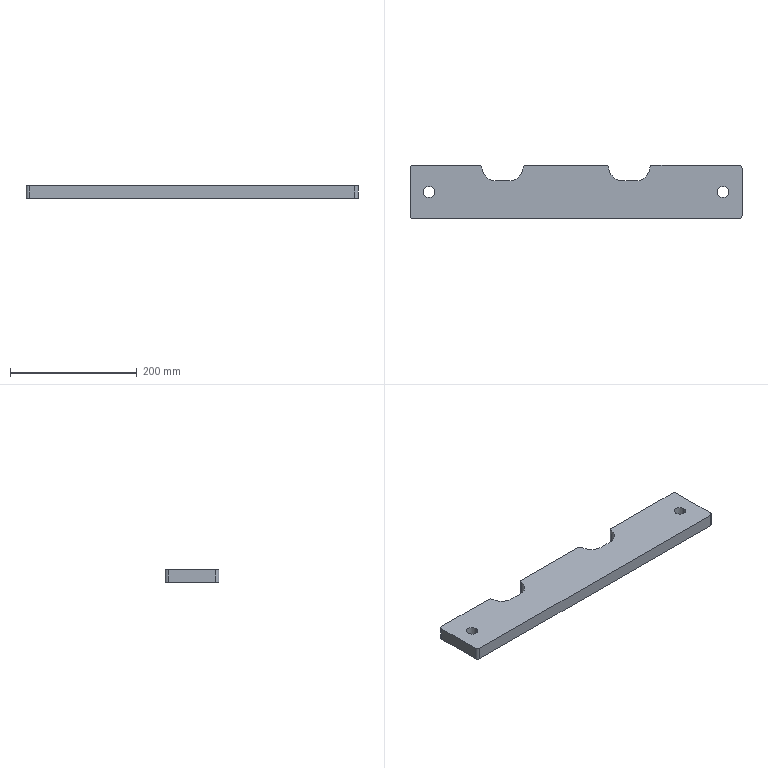Part | SolidWorks | features Extrusion 1 | 1 solid | 26 faces | box 524 x 85 x 20 mm | volume 823491 mm3 | cylinder 16 | plane 10 | commonest cylinder face diameters 10 x8 18 x4 45 x4
STEP:
#1=CARTESIAN_POINT('',(-26200.045,9505.463,20.));
#2=VERTEX_POINT('',#1);
#3=CARTESIAN_POINT('',(-26182.045,9505.463,20.));
#4=VERTEX_POINT('',#3);
#5=CARTESIAN_POINT('',(-26191.045,9505.463,20.));
#6=DIRECTION('',(0.,0.,1.));
#7=DIRECTION('',(1.,0.,0.));
#8=AXIS2_PLACEMENT_3D('',#5,#6,#7);
#9=CIRCLE('',#8,9.);
#10=EDGE_CURVE('',#2,#4,#9,.T.);
#11=ORIENTED_EDGE('',*,*,#10,.T.);
#12=CARTESIAN_POINT('',(-26182.045,9505.463,0.));
#13=VERTEX_POINT('',#12);
#14=CARTESIAN_POINT('',(-26182.045,9505.463,20.));
#15=DIRECTION('',(0.,0.,-1.));
#16=VECTOR('',#15,1000.);
#17=LINE('',#14,#16);
#18=EDGE_CURVE('',#4,#13,#17,.T.);
#19=ORIENTED_EDGE('',*,*,#18,.T.);
#20=CARTESIAN_POINT('',(-26200.045,9505.463,0.));
#21=VERTEX_POINT('',#20);
#22=CARTESIAN_POINT('',(-26191.045,9505.463,0.));
#23=DIRECTION('',(0.,0.,1.));
#24=DIRECTION('',(1.,0.,0.));
#25=AXIS2_PLACEMENT_3D('',#22,#23,#24);
#26=CIRCLE('',#25,9.);
#27=EDGE_CURVE('',#21,#13,#26,.T.);
#28=ORIENTED_EDGE('',*,*,#27,.F.);
#29=CARTESIAN_POINT('',(-26200.045,9505.463,20.));
#30=DIRECTION('',(0.,0.,-1.));
#31=VECTOR('',#30,1000.);
#32=LINE('',#29,#31);
#33=EDGE_CURVE('',#2,#21,#32,.T.);
#34=ORIENTED_EDGE('',*,*,#33,.F.);
#35=EDGE_LOOP('',(#11,#19,#28,#34));
#36=FACE_OUTER_BOUND('',#35,.T.);
#37=CARTESIAN_POINT('',(-26191.045,9505.463,20.));
#38=DIRECTION('',(0.,0.,-1.));
#39=DIRECTION('',(-1.,0.,0.));
#40=AXIS2_PLACEMENT_3D('',#37,#38,#39);
#41=CYLINDRICAL_SURFACE('',#40,9.);
#42=ADVANCED_FACE('',(#36),#41,.F.);
#43=CARTESIAN_POINT('',(-26664.045,9505.463,20.));
#44=VERTEX_POINT('',#43);
#45=CARTESIAN_POINT('',(-26646.045,9505.463,20.));
#46=VERTEX_POINT('',#45);
#47=CARTESIAN_POINT('',(-26655.045,9505.463,20.));
#48=DIRECTION('',(0.,0.,1.));
#49=DIRECTION('',(1.,0.,0.));
#50=AXIS2_PLACEMENT_3D('',#47,#48,#49);
#51=CIRCLE('',#50,9.);
#52=EDGE_CURVE('',#44,#46,#51,.T.);
#53=ORIENTED_EDGE('',*,*,#52,.T.);
#54=CARTESIAN_POINT('',(-26646.045,9505.463,0.));
#55=VERTEX_POINT('',#54);
#56=CARTESIAN_POINT('',(-26646.045,9505.463,20.));
#57=DIRECTION('',(0.,0.,-1.));
#58=VECTOR('',#57,1000.);
#59=LINE('',#56,#58);
#60=EDGE_CURVE('',#46,#55,#59,.T.);
#61=ORIENTED_EDGE('',*,*,#60,.T.);
#62=CARTESIAN_POINT('',(-26664.045,9505.463,0.));
#63=VERTEX_POINT('',#62);
#64=CARTESIAN_POINT('',(-26655.045,9505.463,0.));
#65=DIRECTION('',(0.,0.,1.));
#66=DIRECTION('',(1.,0.,0.));
#67=AXIS2_PLACEMENT_3D('',#64,#65,#66);
#68=CIRCLE('',#67,9.);
#69=EDGE_CURVE('',#63,#55,#68,.T.);
#70=ORIENTED_EDGE('',*,*,#69,.F.);
#71=CARTESIAN_POINT('',(-26664.045,9505.463,20.));
#72=DIRECTION('',(0.,0.,-1.));
#73=VECTOR('',#72,1000.);
#74=LINE('',#71,#73);
#75=EDGE_CURVE('',#44,#63,#74,.T.);
#76=ORIENTED_EDGE('',*,*,#75,.F.);
#77=EDGE_LOOP('',(#53,#61,#70,#76));
#78=FACE_OUTER_BOUND('',#77,.T.);
#79=CARTESIAN_POINT('',(-26655.045,9505.463,20.));
#80=DIRECTION('',(0.,0.,-1.));
#81=DIRECTION('',(-1.,0.,0.));
#82=AXIS2_PLACEMENT_3D('',#79,#80,#81);
#83=CYLINDRICAL_SURFACE('',#82,9.);
#84=ADVANCED_FACE('',(#78),#83,.F.);
#85=ORIENTED_EDGE('',*,*,#52,.F.);
#86=CARTESIAN_POINT('',(-26655.045,9505.463,20.));
#87=DIRECTION('',(0.,0.,1.));
#88=DIRECTION('',(1.,0.,0.));
#89=AXIS2_PLACEMENT_3D('',#86,#87,#88);
#90=CIRCLE('',#89,9.);
#91=EDGE_CURVE('',#46,#44,#90,.T.);
#92=ORIENTED_EDGE('',*,*,#91,.F.);
#93=EDGE_LOOP('',(#85,#92));
#94=FACE_BOUND('',#93,.T.);
#95=CARTESIAN_POINT('',(-26501.659,9547.963,20.));
#96=VERTEX_POINT('',#95);
#97=CARTESIAN_POINT('',(-26506.639,9543.418,20.));
#98=VERTEX_POINT('',#97);
#99=CARTESIAN_POINT('',(-26501.659,9542.963,20.));
#100=DIRECTION('',(0.,0.,1.));
#101=DIRECTION('',(1.,0.,0.));
#102=AXIS2_PLACEMENT_3D('',#99,#100,#101);
#103=CIRCLE('',#102,5.);
#104=EDGE_CURVE('',#96,#98,#103,.T.);
#105=ORIENTED_EDGE('',*,*,#104,.T.);
#106=CARTESIAN_POINT('',(-26529.045,9522.963,20.));
#107=VERTEX_POINT('',#106);
#108=CARTESIAN_POINT('',(-26529.045,9545.463,20.));
#109=DIRECTION('',(0.,0.,-1.));
#110=DIRECTION('',(1.,0.,0.));
#111=AXIS2_PLACEMENT_3D('',#108,#109,#110);
#112=CIRCLE('',#111,22.5);
#113=EDGE_CURVE('',#98,#107,#112,.T.);
#114=ORIENTED_EDGE('',*,*,#113,.T.);
#115=CARTESIAN_POINT('',(-26549.045,9522.963,20.));
#116=VERTEX_POINT('',#115);
#117=CARTESIAN_POINT('',(-26549.045,9522.963,20.));
#118=DIRECTION('',(-1.,0.,0.));
#119=VECTOR('',#118,1000.);
#120=LINE('',#117,#119);
#121=EDGE_CURVE('',#107,#116,#120,.T.);
#122=ORIENTED_EDGE('',*,*,#121,.T.);
#123=CARTESIAN_POINT('',(-26571.452,9543.418,20.));
#124=VERTEX_POINT('',#123);
#125=CARTESIAN_POINT('',(-26549.045,9545.463,20.));
#126=DIRECTION('',(0.,0.,-1.));
#127=DIRECTION('',(1.,0.,0.));
#128=AXIS2_PLACEMENT_3D('',#125,#126,#127);
#129=CIRCLE('',#128,22.5);
#130=EDGE_CURVE('',#116,#124,#129,.T.);
#131=ORIENTED_EDGE('',*,*,#130,.T.);
#132=CARTESIAN_POINT('',(-26576.432,9547.963,20.));
#133=VERTEX_POINT('',#132);
#134=CARTESIAN_POINT('',(-26576.432,9542.963,20.));
#135=DIRECTION('',(0.,0.,1.));
#136=DIRECTION('',(1.,0.,0.));
#137=AXIS2_PLACEMENT_3D('',#134,#135,#136);
#138=CIRCLE('',#137,5.);
#139=EDGE_CURVE('',#124,#133,#138,.T.);
#140=ORIENTED_EDGE('',*,*,#139,.T.);
#141=CARTESIAN_POINT('',(-26680.045,9547.963,20.));
#142=VERTEX_POINT('',#141);
#143=CARTESIAN_POINT('',(-26680.045,9547.963,20.));
#144=DIRECTION('',(-1.,0.,0.));
#145=VECTOR('',#144,1000.);
#146=LINE('',#143,#145);
#147=EDGE_CURVE('',#133,#142,#146,.T.);
#148=ORIENTED_EDGE('',*,*,#147,.T.);
#149=CARTESIAN_POINT('',(-26685.045,9542.963,20.));
#150=VERTEX_POINT('',#149);
#151=CARTESIAN_POINT('',(-26680.045,9542.963,20.));
#152=DIRECTION('',(0.,0.,1.));
#153=DIRECTION('',(1.,0.,0.));
#154=AXIS2_PLACEMENT_3D('',#151,#152,#153);
#155=CIRCLE('',#154,5.);
#156=EDGE_CURVE('',#142,#150,#155,.T.);
#157=ORIENTED_EDGE('',*,*,#156,.T.);
#158=CARTESIAN_POINT('',(-26685.045,9467.963,20.));
#159=VERTEX_POINT('',#158);
#160=CARTESIAN_POINT('',(-26685.045,9467.963,20.));
#161=DIRECTION('',(0.,-1.,0.));
#162=VECTOR('',#161,1000.);
#163=LINE('',#160,#162);
#164=EDGE_CURVE('',#150,#159,#163,.T.);
#165=ORIENTED_EDGE('',*,*,#164,.T.);
#166=CARTESIAN_POINT('',(-26680.045,9462.963,20.));
#167=VERTEX_POINT('',#166);
#168=CARTESIAN_POINT('',(-26680.045,9467.963,20.));
#169=DIRECTION('',(0.,0.,1.));
#170=DIRECTION('',(1.,0.,0.));
#171=AXIS2_PLACEMENT_3D('',#168,#169,#170);
#172=CIRCLE('',#171,5.);
#173=EDGE_CURVE('',#159,#167,#172,.T.);
#174=ORIENTED_EDGE('',*,*,#173,.T.);
#175=CARTESIAN_POINT('',(-26166.045,9462.963,20.));
#176=VERTEX_POINT('',#175);
#177=CARTESIAN_POINT('',(-26166.045,9462.963,20.));
#178=DIRECTION('',(1.,0.,0.));
#179=VECTOR('',#178,1000.);
#180=LINE('',#177,#179);
#181=EDGE_CURVE('',#167,#176,#180,.T.);
#182=ORIENTED_EDGE('',*,*,#181,.T.);
#183=CARTESIAN_POINT('',(-26161.045,9467.963,20.));
#184=VERTEX_POINT('',#183);
#185=CARTESIAN_POINT('',(-26166.045,9467.963,20.));
#186=DIRECTION('',(0.,0.,1.));
#187=DIRECTION('',(1.,0.,0.));
#188=AXIS2_PLACEMENT_3D('',#185,#186,#187);
#189=CIRCLE('',#188,5.);
#190=EDGE_CURVE('',#176,#184,#189,.T.);
#191=ORIENTED_EDGE('',*,*,#190,.T.);
#192=CARTESIAN_POINT('',(-26161.045,9542.963,20.));
#193=VERTEX_POINT('',#192);
#194=CARTESIAN_POINT('',(-26161.045,9467.963,20.));
#195=DIRECTION('',(0.,1.,0.));
#196=VECTOR('',#195,1000.);
#197=LINE('',#194,#196);
#198=EDGE_CURVE('',#184,#193,#197,.T.);
#199=ORIENTED_EDGE('',*,*,#198,.T.);
#200=CARTESIAN_POINT('',(-26166.045,9547.963,20.));
#201=VERTEX_POINT('',#200);
#202=CARTESIAN_POINT('',(-26166.045,9542.963,20.));
#203=DIRECTION('',(0.,0.,1.));
#204=DIRECTION('',(1.,0.,0.));
#205=AXIS2_PLACEMENT_3D('',#202,#203,#204);
#206=CIRCLE('',#205,5.);
#207=EDGE_CURVE('',#193,#201,#206,.T.);
#208=ORIENTED_EDGE('',*,*,#207,.T.);
#209=CARTESIAN_POINT('',(-26301.659,9547.963,20.));
#210=VERTEX_POINT('',#209);
#211=CARTESIAN_POINT('',(-26289.045,9547.963,20.));
#212=DIRECTION('',(-1.,0.,0.));
#213=VECTOR('',#212,1000.);
#214=LINE('',#211,#213);
#215=EDGE_CURVE('',#201,#210,#214,.T.);
#216=ORIENTED_EDGE('',*,*,#215,.T.);
#217=CARTESIAN_POINT('',(-26306.639,9543.418,20.));
#218=VERTEX_POINT('',#217);
#219=CARTESIAN_POINT('',(-26301.659,9542.963,20.));
#220=DIRECTION('',(0.,0.,1.));
#221=DIRECTION('',(1.,0.,0.));
#222=AXIS2_PLACEMENT_3D('',#219,#220,#221);
#223=CIRCLE('',#222,5.);
#224=EDGE_CURVE('',#210,#218,#223,.T.);
#225=ORIENTED_EDGE('',*,*,#224,.T.);
#226=CARTESIAN_POINT('',(-26329.045,9522.963,20.));
#227=VERTEX_POINT('',#226);
#228=CARTESIAN_POINT('',(-26329.045,9545.463,20.));
#229=DIRECTION('',(0.,0.,-1.));
#230=DIRECTION('',(1.,0.,0.));
#231=AXIS2_PLACEMENT_3D('',#228,#229,#230);
#232=CIRCLE('',#231,22.5);
#233=EDGE_CURVE('',#218,#227,#232,.T.);
#234=ORIENTED_EDGE('',*,*,#233,.T.);
#235=CARTESIAN_POINT('',(-26349.045,9522.963,20.));
#236=VERTEX_POINT('',#235);
#237=CARTESIAN_POINT('',(-26349.045,9522.963,20.));
#238=DIRECTION('',(-1.,0.,0.));
#239=VECTOR('',#238,1000.);
#240=LINE('',#237,#239);
#241=EDGE_CURVE('',#227,#236,#240,.T.);
#242=ORIENTED_EDGE('',*,*,#241,.T.);
#243=CARTESIAN_POINT('',(-26371.452,9543.418,20.));
#244=VERTEX_POINT('',#243);
#245=CARTESIAN_POINT('',(-26349.045,9545.463,20.));
#246=DIRECTION('',(0.,0.,-1.));
#247=DIRECTION('',(1.,0.,0.));
#248=AXIS2_PLACEMENT_3D('',#245,#246,#247);
#249=CIRCLE('',#248,22.5);
#250=EDGE_CURVE('',#236,#244,#249,.T.);
#251=ORIENTED_EDGE('',*,*,#250,.T.);
#252=CARTESIAN_POINT('',(-26376.432,9547.963,20.));
#253=VERTEX_POINT('',#252);
#254=CARTESIAN_POINT('',(-26376.432,9542.963,20.));
#255=DIRECTION('',(0.,0.,1.));
#256=DIRECTION('',(1.,0.,0.));
#257=AXIS2_PLACEMENT_3D('',#254,#255,#256);
#258=CIRCLE('',#257,5.);
#259=EDGE_CURVE('',#244,#253,#258,.T.);
#260=ORIENTED_EDGE('',*,*,#259,.T.);
#261=CARTESIAN_POINT('',(-26501.659,9547.963,20.));
#262=DIRECTION('',(-1.,0.,0.));
#263=VECTOR('',#262,1000.);
#264=LINE('',#261,#263);
#265=EDGE_CURVE('',#253,#96,#264,.T.);
#266=ORIENTED_EDGE('',*,*,#265,.T.);
#267=EDGE_LOOP('',(#105,#114,#122,#131,#140,#148,#157,#165,#174,#182,#191,#199,#208,#216,#225,#234,#242,#251,#260,#266));
#268=FACE_OUTER_BOUND('',#267,.T.);
#269=ORIENTED_EDGE('',*,*,#10,.F.);
#270=CARTESIAN_POINT('',(-26191.045,9505.463,20.));
#271=DIRECTION('',(0.,0.,1.));
#272=DIRECTION('',(1.,0.,0.));
#273=AXIS2_PLACEMENT_3D('',#270,#271,#272);
#274=CIRCLE('',#273,9.);
#275=EDGE_CURVE('',#4,#2,#274,.T.);
#276=ORIENTED_EDGE('',*,*,#275,.F.);
#277=EDGE_LOOP('',(#269,#276));
#278=FACE_BOUND('',#277,.T.);
#279=CARTESIAN_POINT('',(-26501.659,9542.963,20.));
#280=DIRECTION('',(0.,0.,1.));
#281=DIRECTION('',(1.,0.,0.));
#282=AXIS2_PLACEMENT_3D('',#279,#280,#281);
#283=PLANE('',#282);
#284=ADVANCED_FACE('',(#94,#268,#278),#283,.T.);
#285=CARTESIAN_POINT('',(-26501.659,9547.963,0.));
#286=VERTEX_POINT('',#285);
#287=CARTESIAN_POINT('',(-26506.639,9543.418,0.));
#288=VERTEX_POINT('',#287);
#289=CARTESIAN_POINT('',(-26501.659,9542.963,0.));
#290=DIRECTION('',(0.,0.,1.));
#291=DIRECTION('',(1.,0.,0.));
#292=AXIS2_PLACEMENT_3D('',#289,#290,#291);
#293=CIRCLE('',#292,5.);
#294=EDGE_CURVE('',#286,#288,#293,.T.);
#295=ORIENTED_EDGE('',*,*,#294,.F.);
#296=CARTESIAN_POINT('',(-26376.432,9547.963,0.));
#297=VERTEX_POINT('',#296);
#298=CARTESIAN_POINT('',(-26501.659,9547.963,0.));
#299=DIRECTION('',(-1.,0.,0.));
#300=VECTOR('',#299,1000.);
#301=LINE('',#298,#300);
#302=EDGE_CURVE('',#297,#286,#301,.T.);
#303=ORIENTED_EDGE('',*,*,#302,.F.);
#304=CARTESIAN_POINT('',(-26371.452,9543.418,0.));
#305=VERTEX_POINT('',#304);
#306=CARTESIAN_POINT('',(-26376.432,9542.963,0.));
#307=DIRECTION('',(0.,0.,1.));
#308=DIRECTION('',(1.,0.,0.));
#309=AXIS2_PLACEMENT_3D('',#306,#307,#308);
#310=CIRCLE('',#309,5.);
#311=EDGE_CURVE('',#305,#297,#310,.T.);
#312=ORIENTED_EDGE('',*,*,#311,.F.);
#313=CARTESIAN_POINT('',(-26349.045,9522.963,0.));
#314=VERTEX_POINT('',#313);
#315=CARTESIAN_POINT('',(-26349.045,9545.463,0.));
#316=DIRECTION('',(0.,0.,-1.));
#317=DIRECTION('',(1.,0.,0.));
#318=AXIS2_PLACEMENT_3D('',#315,#316,#317);
#319=CIRCLE('',#318,22.5);
#320=EDGE_CURVE('',#314,#305,#319,.T.);
#321=ORIENTED_EDGE('',*,*,#320,.F.);
#322=CARTESIAN_POINT('',(-26329.045,9522.963,0.));
#323=VERTEX_POINT('',#322);
#324=CARTESIAN_POINT('',(-26349.045,9522.963,0.));
#325=DIRECTION('',(-1.,0.,0.));
#326=VECTOR('',#325,1000.);
#327=LINE('',#324,#326);
#328=EDGE_CURVE('',#323,#314,#327,.T.);
#329=ORIENTED_EDGE('',*,*,#328,.F.);
#330=CARTESIAN_POINT('',(-26306.639,9543.418,0.));
#331=VERTEX_POINT('',#330);
#332=CARTESIAN_POINT('',(-26329.045,9545.463,0.));
#333=DIRECTION('',(0.,0.,-1.));
#334=DIRECTION('',(1.,0.,0.));
#335=AXIS2_PLACEMENT_3D('',#332,#333,#334);
#336=CIRCLE('',#335,22.5);
#337=EDGE_CURVE('',#331,#323,#336,.T.);
#338=ORIENTED_EDGE('',*,*,#337,.F.);
#339=CARTESIAN_POINT('',(-26301.659,9547.963,0.));
#340=VERTEX_POINT('',#339);
#341=CARTESIAN_POINT('',(-26301.659,9542.963,0.));
#342=DIRECTION('',(0.,0.,1.));
#343=DIRECTION('',(1.,0.,0.));
#344=AXIS2_PLACEMENT_3D('',#341,#342,#343);
#345=CIRCLE('',#344,5.);
#346=EDGE_CURVE('',#340,#331,#345,.T.);
#347=ORIENTED_EDGE('',*,*,#346,.F.);
#348=CARTESIAN_POINT('',(-26166.045,9547.963,0.));
#349=VERTEX_POINT('',#348);
#350=CARTESIAN_POINT('',(-26301.659,9547.963,0.));
#351=DIRECTION('',(-1.,0.,0.));
#352=VECTOR('',#351,1000.);
#353=LINE('',#350,#352);
#354=EDGE_CURVE('',#349,#340,#353,.T.);
#355=ORIENTED_EDGE('',*,*,#354,.F.);
#356=CARTESIAN_POINT('',(-26161.045,9542.963,0.));
#357=VERTEX_POINT('',#356);
#358=CARTESIAN_POINT('',(-26166.045,9542.963,0.));
#359=DIRECTION('',(0.,0.,1.));
#360=DIRECTION('',(1.,0.,0.));
#361=AXIS2_PLACEMENT_3D('',#358,#359,#360);
#362=CIRCLE('',#361,5.);
#363=EDGE_CURVE('',#357,#349,#362,.T.);
#364=ORIENTED_EDGE('',*,*,#363,.F.);
#365=CARTESIAN_POINT('',(-26161.045,9467.963,0.));
#366=VERTEX_POINT('',#365);
#367=CARTESIAN_POINT('',(-26161.045,9467.963,0.));
#368=DIRECTION('',(0.,1.,0.));
#369=VECTOR('',#368,1000.);
#370=LINE('',#367,#369);
#371=EDGE_CURVE('',#366,#357,#370,.T.);
#372=ORIENTED_EDGE('',*,*,#371,.F.);
#373=CARTESIAN_POINT('',(-26166.045,9462.963,0.));
#374=VERTEX_POINT('',#373);
#375=CARTESIAN_POINT('',(-26166.045,9467.963,0.));
#376=DIRECTION('',(0.,0.,1.));
#377=DIRECTION('',(1.,0.,0.));
#378=AXIS2_PLACEMENT_3D('',#375,#376,#377);
#379=CIRCLE('',#378,5.);
#380=EDGE_CURVE('',#374,#366,#379,.T.);
#381=ORIENTED_EDGE('',*,*,#380,.F.);
#382=CARTESIAN_POINT('',(-26680.045,9462.963,0.));
#383=VERTEX_POINT('',#382);
#384=CARTESIAN_POINT('',(-26166.045,9462.963,0.));
#385=DIRECTION('',(1.,0.,0.));
#386=VECTOR('',#385,1000.);
#387=LINE('',#384,#386);
#388=EDGE_CURVE('',#383,#374,#387,.T.);
#389=ORIENTED_EDGE('',*,*,#388,.F.);
#390=CARTESIAN_POINT('',(-26685.045,9467.963,0.));
#391=VERTEX_POINT('',#390);
#392=CARTESIAN_POINT('',(-26680.045,9467.963,0.));
#393=DIRECTION('',(0.,0.,1.));
#394=DIRECTION('',(1.,0.,0.));
#395=AXIS2_PLACEMENT_3D('',#392,#393,#394);
#396=CIRCLE('',#395,5.);
#397=EDGE_CURVE('',#391,#383,#396,.T.);
#398=ORIENTED_EDGE('',*,*,#397,.F.);
#399=CARTESIAN_POINT('',(-26685.045,9542.963,0.));
#400=VERTEX_POINT('',#399);
#401=CARTESIAN_POINT('',(-26685.045,9467.963,0.));
#402=DIRECTION('',(0.,-1.,0.));
#403=VECTOR('',#402,1000.);
#404=LINE('',#401,#403);
#405=EDGE_CURVE('',#400,#391,#404,.T.);
#406=ORIENTED_EDGE('',*,*,#405,.F.);
#407=CARTESIAN_POINT('',(-26680.045,9547.963,0.));
#408=VERTEX_POINT('',#407);
#409=CARTESIAN_POINT('',(-26680.045,9542.963,0.));
#410=DIRECTION('',(0.,0.,1.));
#411=DIRECTION('',(1.,0.,0.));
#412=AXIS2_PLACEMENT_3D('',#409,#410,#411);
#413=CIRCLE('',#412,5.);
#414=EDGE_CURVE('',#408,#400,#413,.T.);
#415=ORIENTED_EDGE('',*,*,#414,.F.);
#416=CARTESIAN_POINT('',(-26576.432,9547.963,0.));
#417=VERTEX_POINT('',#416);
#418=CARTESIAN_POINT('',(-26680.045,9547.963,0.));
#419=DIRECTION('',(-1.,0.,0.));
#420=VECTOR('',#419,1000.);
#421=LINE('',#418,#420);
#422=EDGE_CURVE('',#417,#408,#421,.T.);
#423=ORIENTED_EDGE('',*,*,#422,.F.);
#424=CARTESIAN_POINT('',(-26571.452,9543.418,0.));
#425=VERTEX_POINT('',#424);
#426=CARTESIAN_POINT('',(-26576.432,9542.963,0.));
#427=DIRECTION('',(0.,0.,1.));
#428=DIRECTION('',(1.,0.,0.));
#429=AXIS2_PLACEMENT_3D('',#426,#427,#428);
#430=CIRCLE('',#429,5.);
#431=EDGE_CURVE('',#425,#417,#430,.T.);
#432=ORIENTED_EDGE('',*,*,#431,.F.);
#433=CARTESIAN_POINT('',(-26549.045,9522.963,0.));
#434=VERTEX_POINT('',#433);
#435=CARTESIAN_POINT('',(-26549.045,9545.463,0.));
#436=DIRECTION('',(0.,0.,-1.));
#437=DIRECTION('',(1.,0.,0.));
#438=AXIS2_PLACEMENT_3D('',#435,#436,#437);
#439=CIRCLE('',#438,22.5);
#440=EDGE_CURVE('',#434,#425,#439,.T.);
#441=ORIENTED_EDGE('',*,*,#440,.F.);
#442=CARTESIAN_POINT('',(-26529.045,9522.963,0.));
#443=VERTEX_POINT('',#442);
#444=CARTESIAN_POINT('',(-26549.045,9522.963,0.));
#445=DIRECTION('',(-1.,0.,0.));
#446=VECTOR('',#445,1000.);
#447=LINE('',#444,#446);
#448=EDGE_CURVE('',#443,#434,#447,.T.);
#449=ORIENTED_EDGE('',*,*,#448,.F.);
#450=CARTESIAN_POINT('',(-26529.045,9545.463,0.));
#451=DIRECTION('',(0.,0.,-1.));
#452=DIRECTION('',(1.,0.,0.));
#453=AXIS2_PLACEMENT_3D('',#450,#451,#452);
#454=CIRCLE('',#453,22.5);
#455=EDGE_CURVE('',#288,#443,#454,.T.);
#456=ORIENTED_EDGE('',*,*,#455,.F.);
#457=EDGE_LOOP('',(#295,#303,#312,#321,#329,#338,#347,#355,#364,#372,#381,#389,#398,#406,#415,#423,#432,#441,#449,#456));
#458=FACE_OUTER_BOUND('',#457,.T.);
#459=ORIENTED_EDGE('',*,*,#69,.T.);
#460=CARTESIAN_POINT('',(-26655.045,9505.463,0.));
#461=DIRECTION('',(0.,0.,1.));
#462=DIRECTION('',(1.,0.,0.));
#463=AXIS2_PLACEMENT_3D('',#460,#461,#462);
#464=CIRCLE('',#463,9.);
#465=EDGE_CURVE('',#55,#63,#464,.T.);
#466=ORIENTED_EDGE('',*,*,#465,.T.);
#467=EDGE_LOOP('',(#459,#466));
#468=FACE_BOUND('',#467,.T.);
#469=ORIENTED_EDGE('',*,*,#27,.T.);
#470=CARTESIAN_POINT('',(-26191.045,9505.463,0.));
#471=DIRECTION('',(0.,0.,1.));
#472=DIRECTION('',(1.,0.,0.));
#473=AXIS2_PLACEMENT_3D('',#470,#471,#472);
#474=CIRCLE('',#473,9.);
#475=EDGE_CURVE('',#13,#21,#474,.T.);
#476=ORIENTED_EDGE('',*,*,#475,.T.);
#477=EDGE_LOOP('',(#469,#476));
#478=FACE_BOUND('',#477,.T.);
#479=CARTESIAN_POINT('',(-26501.659,9542.963,0.));
#480=DIRECTION('',(0.,0.,1.));
#481=DIRECTION('',(1.,0.,0.));
#482=AXIS2_PLACEMENT_3D('',#479,#480,#481);
#483=PLANE('',#482);
#484=ADVANCED_FACE('',(#458,#468,#478),#483,.F.);
#485=ORIENTED_EDGE('',*,*,#294,.T.);
#486=CARTESIAN_POINT('',(-26506.639,9543.418,20.));
#487=DIRECTION('',(0.,0.,-1.));
#488=VECTOR('',#487,1000.);
#489=LINE('',#486,#488);
#490=EDGE_CURVE('',#98,#288,#489,.T.);
#491=ORIENTED_EDGE('',*,*,#490,.F.);
#492=ORIENTED_EDGE('',*,*,#104,.F.);
#493=CARTESIAN_POINT('',(-26501.659,9547.963,20.));
#494=DIRECTION('',(0.,0.,-1.));
#495=VECTOR('',#494,1000.);
#496=LINE('',#493,#495);
#497=EDGE_CURVE('',#96,#286,#496,.T.);
#498=ORIENTED_EDGE('',*,*,#497,.T.);
#499=EDGE_LOOP('',(#485,#491,#492,#498));
#500=FACE_OUTER_BOUND('',#499,.T.);
#501=CARTESIAN_POINT('',(-26501.659,9542.963,20.));
#502=DIRECTION('',(0.,0.,-1.));
#503=DIRECTION('',(-1.,0.,0.));
#504=AXIS2_PLACEMENT_3D('',#501,#502,#503);
#505=CYLINDRICAL_SURFACE('',#504,5.);
#506=ADVANCED_FACE('',(#500),#505,.T.);
#507=ORIENTED_EDGE('',*,*,#455,.T.);
#508=CARTESIAN_POINT('',(-26529.045,9522.963,20.));
#509=DIRECTION('',(0.,0.,-1.));
#510=VECTOR('',#509,1000.);
#511=LINE('',#508,#510);
#512=EDGE_CURVE('',#107,#443,#511,.T.);
#513=ORIENTED_EDGE('',*,*,#512,.F.);
#514=ORIENTED_EDGE('',*,*,#113,.F.);
#515=ORIENTED_EDGE('',*,*,#490,.T.);
#516=EDGE_LOOP('',(#507,#513,#514,#515));
#517=FACE_OUTER_BOUND('',#516,.T.);
#518=CARTESIAN_POINT('',(-26529.045,9545.463,20.));
#519=DIRECTION('',(0.,0.,-1.));
#520=DIRECTION('',(-1.,0.,0.));
#521=AXIS2_PLACEMENT_3D('',#518,#519,#520);
#522=CYLINDRICAL_SURFACE('',#521,22.5);
#523=ADVANCED_FACE('',(#517),#522,.F.);
#524=ORIENTED_EDGE('',*,*,#448,.T.);
#525=CARTESIAN_POINT('',(-26549.045,9522.963,20.));
#526=DIRECTION('',(0.,0.,-1.));
#527=VECTOR('',#526,1000.);
#528=LINE('',#525,#527);
#529=EDGE_CURVE('',#116,#434,#528,.T.);
#530=ORIENTED_EDGE('',*,*,#529,.F.);
#531=ORIENTED_EDGE('',*,*,#121,.F.);
#532=ORIENTED_EDGE('',*,*,#512,.T.);
#533=EDGE_LOOP('',(#524,#530,#531,#532));
#534=FACE_OUTER_BOUND('',#533,.T.);
#535=CARTESIAN_POINT('',(-26549.045,9522.963,20.));
#536=DIRECTION('',(0.,-1.,0.));
#537=DIRECTION('',(0.,0.,-1.));
#538=AXIS2_PLACEMENT_3D('',#535,#536,#537);
#539=PLANE('',#538);
#540=ADVANCED_FACE('',(#534),#539,.F.);
#541=ORIENTED_EDGE('',*,*,#440,.T.);
#542=CARTESIAN_POINT('',(-26571.452,9543.418,20.));
#543=DIRECTION('',(0.,0.,-1.));
#544=VECTOR('',#543,1000.);
#545=LINE('',#542,#544);
#546=EDGE_CURVE('',#124,#425,#545,.T.);
#547=ORIENTED_EDGE('',*,*,#546,.F.);
#548=ORIENTED_EDGE('',*,*,#130,.F.);
#549=ORIENTED_EDGE('',*,*,#529,.T.);
#550=EDGE_LOOP('',(#541,#547,#548,#549));
#551=FACE_OUTER_BOUND('',#550,.T.);
#552=CARTESIAN_POINT('',(-26549.045,9545.463,20.));
#553=DIRECTION('',(0.,0.,-1.));
#554=DIRECTION('',(-1.,0.,0.));
#555=AXIS2_PLACEMENT_3D('',#552,#553,#554);
#556=CYLINDRICAL_SURFACE('',#555,22.5);
#557=ADVANCED_FACE('',(#551),#556,.F.);
#558=ORIENTED_EDGE('',*,*,#431,.T.);
#559=CARTESIAN_POINT('',(-26576.432,9547.963,20.));
#560=DIRECTION('',(0.,0.,-1.));
#561=VECTOR('',#560,1000.);
#562=LINE('',#559,#561);
#563=EDGE_CURVE('',#133,#417,#562,.T.);
#564=ORIENTED_EDGE('',*,*,#563,.F.);
#565=ORIENTED_EDGE('',*,*,#139,.F.);
#566=ORIENTED_EDGE('',*,*,#546,.T.);
#567=EDGE_LOOP('',(#558,#564,#565,#566));
#568=FACE_OUTER_BOUND('',#567,.T.);
#569=CARTESIAN_POINT('',(-26576.432,9542.963,20.));
#570=DIRECTION('',(0.,0.,-1.));
#571=DIRECTION('',(-1.,0.,0.));
#572=AXIS2_PLACEMENT_3D('',#569,#570,#571);
#573=CYLINDRICAL_SURFACE('',#572,5.);
#574=ADVANCED_FACE('',(#568),#573,.T.);
#575=ORIENTED_EDGE('',*,*,#422,.T.);
#576=CARTESIAN_POINT('',(-26680.045,9547.963,20.));
#577=DIRECTION('',(0.,0.,-1.));
#578=VECTOR('',#577,1000.);
#579=LINE('',#576,#578);
#580=EDGE_CURVE('',#142,#408,#579,.T.);
#581=ORIENTED_EDGE('',*,*,#580,.F.);
#582=ORIENTED_EDGE('',*,*,#147,.F.);
#583=ORIENTED_EDGE('',*,*,#563,.T.);
#584=EDGE_LOOP('',(#575,#581,#582,#583));
#585=FACE_OUTER_BOUND('',#584,.T.);
#586=CARTESIAN_POINT('',(-26680.045,9547.963,20.));
#587=DIRECTION('',(0.,-1.,0.));
#588=DIRECTION('',(0.,0.,-1.));
#589=AXIS2_PLACEMENT_3D('',#586,#587,#588);
#590=PLANE('',#589);
#591=ADVANCED_FACE('',(#585),#590,.F.);
#592=ORIENTED_EDGE('',*,*,#414,.T.);
#593=CARTESIAN_POINT('',(-26685.045,9542.963,20.));
#594=DIRECTION('',(0.,0.,-1.));
#595=VECTOR('',#594,1000.);
#596=LINE('',#593,#595);
#597=EDGE_CURVE('',#150,#400,#596,.T.);
#598=ORIENTED_EDGE('',*,*,#597,.F.);
#599=ORIENTED_EDGE('',*,*,#156,.F.);
#600=ORIENTED_EDGE('',*,*,#580,.T.);
#601=EDGE_LOOP('',(#592,#598,#599,#600));
#602=FACE_OUTER_BOUND('',#601,.T.);
#603=CARTESIAN_POINT('',(-26680.045,9542.963,20.));
#604=DIRECTION('',(0.,0.,-1.));
#605=DIRECTION('',(-1.,0.,0.));
#606=AXIS2_PLACEMENT_3D('',#603,#604,#605);
#607=CYLINDRICAL_SURFACE('',#606,5.);
#608=ADVANCED_FACE('',(#602),#607,.T.);
#609=ORIENTED_EDGE('',*,*,#405,.T.);
#610=CARTESIAN_POINT('',(-26685.045,9467.963,20.));
#611=DIRECTION('',(0.,0.,-1.));
#612=VECTOR('',#611,1000.);
#613=LINE('',#610,#612);
#614=EDGE_CURVE('',#159,#391,#613,.T.);
#615=ORIENTED_EDGE('',*,*,#614,.F.);
#616=ORIENTED_EDGE('',*,*,#164,.F.);
#617=ORIENTED_EDGE('',*,*,#597,.T.);
#618=EDGE_LOOP('',(#609,#615,#616,#617));
#619=FACE_OUTER_BOUND('',#618,.T.);
#620=CARTESIAN_POINT('',(-26685.045,9467.963,20.));
#621=DIRECTION('',(1.,0.,0.));
#622=DIRECTION('',(0.,0.,-1.));
#623=AXIS2_PLACEMENT_3D('',#620,#621,#622);
#624=PLANE('',#623);
#625=ADVANCED_FACE('',(#619),#624,.F.);
#626=ORIENTED_EDGE('',*,*,#397,.T.);
#627=CARTESIAN_POINT('',(-26680.045,9462.963,20.));
#628=DIRECTION('',(0.,0.,-1.));
#629=VECTOR('',#628,1000.);
#630=LINE('',#627,#629);
#631=EDGE_CURVE('',#167,#383,#630,.T.);
#632=ORIENTED_EDGE('',*,*,#631,.F.);
#633=ORIENTED_EDGE('',*,*,#173,.F.);
#634=ORIENTED_EDGE('',*,*,#614,.T.);
#635=EDGE_LOOP('',(#626,#632,#633,#634));
#636=FACE_OUTER_BOUND('',#635,.T.);
#637=CARTESIAN_POINT('',(-26680.045,9467.963,20.));
#638=DIRECTION('',(0.,0.,-1.));
#639=DIRECTION('',(-1.,0.,0.));
#640=AXIS2_PLACEMENT_3D('',#637,#638,#639);
#641=CYLINDRICAL_SURFACE('',#640,5.);
#642=ADVANCED_FACE('',(#636),#641,.T.);
#643=ORIENTED_EDGE('',*,*,#388,.T.);
#644=CARTESIAN_POINT('',(-26166.045,9462.963,20.));
#645=DIRECTION('',(0.,0.,-1.));
#646=VECTOR('',#645,1000.);
#647=LINE('',#644,#646);
#648=EDGE_CURVE('',#176,#374,#647,.T.);
#649=ORIENTED_EDGE('',*,*,#648,.F.);
#650=ORIENTED_EDGE('',*,*,#181,.F.);
#651=ORIENTED_EDGE('',*,*,#631,.T.);
#652=EDGE_LOOP('',(#643,#649,#650,#651));
#653=FACE_OUTER_BOUND('',#652,.T.);
#654=CARTESIAN_POINT('',(-26166.045,9462.963,20.));
#655=DIRECTION('',(0.,1.,0.));
#656=DIRECTION('',(-1.,0.,0.));
#657=AXIS2_PLACEMENT_3D('',#654,#655,#656);
#658=PLANE('',#657);
#659=ADVANCED_FACE('',(#653),#658,.F.);
#660=ORIENTED_EDGE('',*,*,#380,.T.);
#661=CARTESIAN_POINT('',(-26161.045,9467.963,20.));
#662=DIRECTION('',(0.,0.,-1.));
#663=VECTOR('',#662,1000.);
#664=LINE('',#661,#663);
#665=EDGE_CURVE('',#184,#366,#664,.T.);
#666=ORIENTED_EDGE('',*,*,#665,.F.);
#667=ORIENTED_EDGE('',*,*,#190,.F.);
#668=ORIENTED_EDGE('',*,*,#648,.T.);
#669=EDGE_LOOP('',(#660,#666,#667,#668));
#670=FACE_OUTER_BOUND('',#669,.T.);
#671=CARTESIAN_POINT('',(-26166.045,9467.963,20.));
#672=DIRECTION('',(0.,0.,-1.));
#673=DIRECTION('',(-1.,0.,0.));
#674=AXIS2_PLACEMENT_3D('',#671,#672,#673);
#675=CYLINDRICAL_SURFACE('',#674,5.);
#676=ADVANCED_FACE('',(#670),#675,.T.);
#677=ORIENTED_EDGE('',*,*,#371,.T.);
#678=CARTESIAN_POINT('',(-26161.045,9542.963,20.));
#679=DIRECTION('',(0.,0.,-1.));
#680=VECTOR('',#679,1000.);
#681=LINE('',#678,#680);
#682=EDGE_CURVE('',#193,#357,#681,.T.);
#683=ORIENTED_EDGE('',*,*,#682,.F.);
#684=ORIENTED_EDGE('',*,*,#198,.F.);
#685=ORIENTED_EDGE('',*,*,#665,.T.);
#686=EDGE_LOOP('',(#677,#683,#684,#685));
#687=FACE_OUTER_BOUND('',#686,.T.);
#688=CARTESIAN_POINT('',(-26161.045,9467.963,20.));
#689=DIRECTION('',(-1.,0.,0.));
#690=DIRECTION('',(0.,0.,1.));
#691=AXIS2_PLACEMENT_3D('',#688,#689,#690);
#692=PLANE('',#691);
#693=ADVANCED_FACE('',(#687),#692,.F.);
#694=ORIENTED_EDGE('',*,*,#363,.T.);
#695=CARTESIAN_POINT('',(-26166.045,9547.963,20.));
#696=DIRECTION('',(0.,0.,-1.));
#697=VECTOR('',#696,1000.);
#698=LINE('',#695,#697);
#699=EDGE_CURVE('',#201,#349,#698,.T.);
#700=ORIENTED_EDGE('',*,*,#699,.F.);
#701=ORIENTED_EDGE('',*,*,#207,.F.);
#702=ORIENTED_EDGE('',*,*,#682,.T.);
#703=EDGE_LOOP('',(#694,#700,#701,#702));
#704=FACE_OUTER_BOUND('',#703,.T.);
#705=CARTESIAN_POINT('',(-26166.045,9542.963,20.));
#706=DIRECTION('',(0.,0.,-1.));
#707=DIRECTION('',(-1.,0.,0.));
#708=AXIS2_PLACEMENT_3D('',#705,#706,#707);
#709=CYLINDRICAL_SURFACE('',#708,5.);
#710=ADVANCED_FACE('',(#704),#709,.T.);
#711=ORIENTED_EDGE('',*,*,#354,.T.);
#712=CARTESIAN_POINT('',(-26301.659,9547.963,20.));
#713=DIRECTION('',(0.,0.,-1.));
#714=VECTOR('',#713,1000.);
#715=LINE('',#712,#714);
#716=EDGE_CURVE('',#210,#340,#715,.T.);
#717=ORIENTED_EDGE('',*,*,#716,.F.);
#718=ORIENTED_EDGE('',*,*,#215,.F.);
#719=ORIENTED_EDGE('',*,*,#699,.T.);
#720=EDGE_LOOP('',(#711,#717,#718,#719));
#721=FACE_OUTER_BOUND('',#720,.T.);
#722=CARTESIAN_POINT('',(-26301.659,9547.963,20.));
#723=DIRECTION('',(0.,-1.,0.));
#724=DIRECTION('',(0.,0.,-1.));
#725=AXIS2_PLACEMENT_3D('',#722,#723,#724);
#726=PLANE('',#725);
#727=ADVANCED_FACE('',(#721),#726,.F.);
#728=ORIENTED_EDGE('',*,*,#346,.T.);
#729=CARTESIAN_POINT('',(-26306.639,9543.418,20.));
#730=DIRECTION('',(0.,0.,-1.));
#731=VECTOR('',#730,1000.);
#732=LINE('',#729,#731);
#733=EDGE_CURVE('',#218,#331,#732,.T.);
#734=ORIENTED_EDGE('',*,*,#733,.F.);
#735=ORIENTED_EDGE('',*,*,#224,.F.);
#736=ORIENTED_EDGE('',*,*,#716,.T.);
#737=EDGE_LOOP('',(#728,#734,#735,#736));
#738=FACE_OUTER_BOUND('',#737,.T.);
#739=CARTESIAN_POINT('',(-26301.659,9542.963,20.));
#740=DIRECTION('',(0.,0.,-1.));
#741=DIRECTION('',(-1.,0.,0.));
#742=AXIS2_PLACEMENT_3D('',#739,#740,#741);
#743=CYLINDRICAL_SURFACE('',#742,5.);
#744=ADVANCED_FACE('',(#738),#743,.T.);
#745=ORIENTED_EDGE('',*,*,#337,.T.);
#746=CARTESIAN_POINT('',(-26329.045,9522.963,20.));
#747=DIRECTION('',(0.,0.,-1.));
#748=VECTOR('',#747,1000.);
#749=LINE('',#746,#748);
#750=EDGE_CURVE('',#227,#323,#749,.T.);
#751=ORIENTED_EDGE('',*,*,#750,.F.);
#752=ORIENTED_EDGE('',*,*,#233,.F.);
#753=ORIENTED_EDGE('',*,*,#733,.T.);
#754=EDGE_LOOP('',(#745,#751,#752,#753));
#755=FACE_OUTER_BOUND('',#754,.T.);
#756=CARTESIAN_POINT('',(-26329.045,9545.463,20.));
#757=DIRECTION('',(0.,0.,-1.));
#758=DIRECTION('',(-1.,0.,0.));
#759=AXIS2_PLACEMENT_3D('',#756,#757,#758);
#760=CYLINDRICAL_SURFACE('',#759,22.5);
#761=ADVANCED_FACE('',(#755),#760,.F.);
#762=ORIENTED_EDGE('',*,*,#328,.T.);
#763=CARTESIAN_POINT('',(-26349.045,9522.963,20.));
#764=DIRECTION('',(0.,0.,-1.));
#765=VECTOR('',#764,1000.);
#766=LINE('',#763,#765);
#767=EDGE_CURVE('',#236,#314,#766,.T.);
#768=ORIENTED_EDGE('',*,*,#767,.F.);
#769=ORIENTED_EDGE('',*,*,#241,.F.);
#770=ORIENTED_EDGE('',*,*,#750,.T.);
#771=EDGE_LOOP('',(#762,#768,#769,#770));
#772=FACE_OUTER_BOUND('',#771,.T.);
#773=CARTESIAN_POINT('',(-26349.045,9522.963,20.));
#774=DIRECTION('',(0.,-1.,0.));
#775=DIRECTION('',(0.,0.,-1.));
#776=AXIS2_PLACEMENT_3D('',#773,#774,#775);
#777=PLANE('',#776);
#778=ADVANCED_FACE('',(#772),#777,.F.);
#779=ORIENTED_EDGE('',*,*,#320,.T.);
#780=CARTESIAN_POINT('',(-26371.452,9543.418,20.));
#781=DIRECTION('',(0.,0.,-1.));
#782=VECTOR('',#781,1000.);
#783=LINE('',#780,#782);
#784=EDGE_CURVE('',#244,#305,#783,.T.);
#785=ORIENTED_EDGE('',*,*,#784,.F.);
#786=ORIENTED_EDGE('',*,*,#250,.F.);
#787=ORIENTED_EDGE('',*,*,#767,.T.);
#788=EDGE_LOOP('',(#779,#785,#786,#787));
#789=FACE_OUTER_BOUND('',#788,.T.);
#790=CARTESIAN_POINT('',(-26349.045,9545.463,20.));
#791=DIRECTION('',(0.,0.,-1.));
#792=DIRECTION('',(-1.,0.,0.));
#793=AXIS2_PLACEMENT_3D('',#790,#791,#792);
#794=CYLINDRICAL_SURFACE('',#793,22.5);
#795=ADVANCED_FACE('',(#789),#794,.F.);
#796=ORIENTED_EDGE('',*,*,#311,.T.);
#797=CARTESIAN_POINT('',(-26376.432,9547.963,20.));
#798=DIRECTION('',(0.,0.,-1.));
#799=VECTOR('',#798,1000.);
#800=LINE('',#797,#799);
#801=EDGE_CURVE('',#253,#297,#800,.T.);
#802=ORIENTED_EDGE('',*,*,#801,.F.);
#803=ORIENTED_EDGE('',*,*,#259,.F.);
#804=ORIENTED_EDGE('',*,*,#784,.T.);
#805=EDGE_LOOP('',(#796,#802,#803,#804));
#806=FACE_OUTER_BOUND('',#805,.T.);
#807=CARTESIAN_POINT('',(-26376.432,9542.963,20.));
#808=DIRECTION('',(0.,0.,-1.));
#809=DIRECTION('',(-1.,0.,0.));
#810=AXIS2_PLACEMENT_3D('',#807,#808,#809);
#811=CYLINDRICAL_SURFACE('',#810,5.);
#812=ADVANCED_FACE('',(#806),#811,.T.);
#813=ORIENTED_EDGE('',*,*,#302,.T.);
#814=ORIENTED_EDGE('',*,*,#497,.F.);
#815=ORIENTED_EDGE('',*,*,#265,.F.);
#816=ORIENTED_EDGE('',*,*,#801,.T.);
#817=EDGE_LOOP('',(#813,#814,#815,#816));
#818=FACE_OUTER_BOUND('',#817,.T.);
#819=CARTESIAN_POINT('',(-26501.659,9547.963,20.));
#820=DIRECTION('',(0.,-1.,0.));
#821=DIRECTION('',(0.,0.,-1.));
#822=AXIS2_PLACEMENT_3D('',#819,#820,#821);
#823=PLANE('',#822);
#824=ADVANCED_FACE('',(#818),#823,.F.);
#825=ORIENTED_EDGE('',*,*,#60,.F.);
#826=ORIENTED_EDGE('',*,*,#91,.T.);
#827=ORIENTED_EDGE('',*,*,#75,.T.);
#828=ORIENTED_EDGE('',*,*,#465,.F.);
#829=EDGE_LOOP('',(#825,#826,#827,#828));
#830=FACE_OUTER_BOUND('',#829,.T.);
#831=CARTESIAN_POINT('',(-26655.045,9505.463,20.));
#832=DIRECTION('',(0.,0.,-1.));
#833=DIRECTION('',(-1.,0.,0.));
#834=AXIS2_PLACEMENT_3D('',#831,#832,#833);
#835=CYLINDRICAL_SURFACE('',#834,9.);
#836=ADVANCED_FACE('',(#830),#835,.F.);
#837=ORIENTED_EDGE('',*,*,#18,.F.);
#838=ORIENTED_EDGE('',*,*,#275,.T.);
#839=ORIENTED_EDGE('',*,*,#33,.T.);
#840=ORIENTED_EDGE('',*,*,#475,.F.);
#841=EDGE_LOOP('',(#837,#838,#839,#840));
#842=FACE_OUTER_BOUND('',#841,.T.);
#843=CARTESIAN_POINT('',(-26191.045,9505.463,20.));
#844=DIRECTION('',(0.,0.,-1.));
#845=DIRECTION('',(-1.,0.,0.));
#846=AXIS2_PLACEMENT_3D('',#843,#844,#845);
#847=CYLINDRICAL_SURFACE('',#846,9.);
#848=ADVANCED_FACE('',(#842),#847,.F.);
#849=CLOSED_SHELL('',(#42,#84,#284,#484,#506,#523,#540,#557,#574,#591,#608,#625,#642,#659,#676,#693,#710,#727,#744,#761,#778,#795,#812,#824,#836,#848));
#850=MANIFOLD_SOLID_BREP('',#849);
#851=CARTESIAN_POINT('',(0.,0.,0.));
#852=DIRECTION('',(0.,0.,1.));
#853=DIRECTION('',(1.,0.,0.));
#854=AXIS2_PLACEMENT_3D('',#851,#852,#853);
#855=(LENGTH_UNIT()NAMED_UNIT(*)SI_UNIT(.MILLI.,.METRE.));
#856=UNCERTAINTY_MEASURE_WITH_UNIT(LENGTH_MEASURE(0.00001),#855,'','');
#857=(NAMED_UNIT(*)PLANE_ANGLE_UNIT()SI_UNIT($,.RADIAN.));
#858=(NAMED_UNIT(*)SI_UNIT($,.STERADIAN.)SOLID_ANGLE_UNIT());
#859=(GEOMETRIC_REPRESENTATION_CONTEXT(3)GLOBAL_UNCERTAINTY_ASSIGNED_CONTEXT((#856))GLOBAL_UNIT_ASSIGNED_CONTEXT((#855,#857,#858))REPRESENTATION_CONTEXT('',''));
#860=ADVANCED_BREP_SHAPE_REPRESENTATION('',(#850,#854),#859);